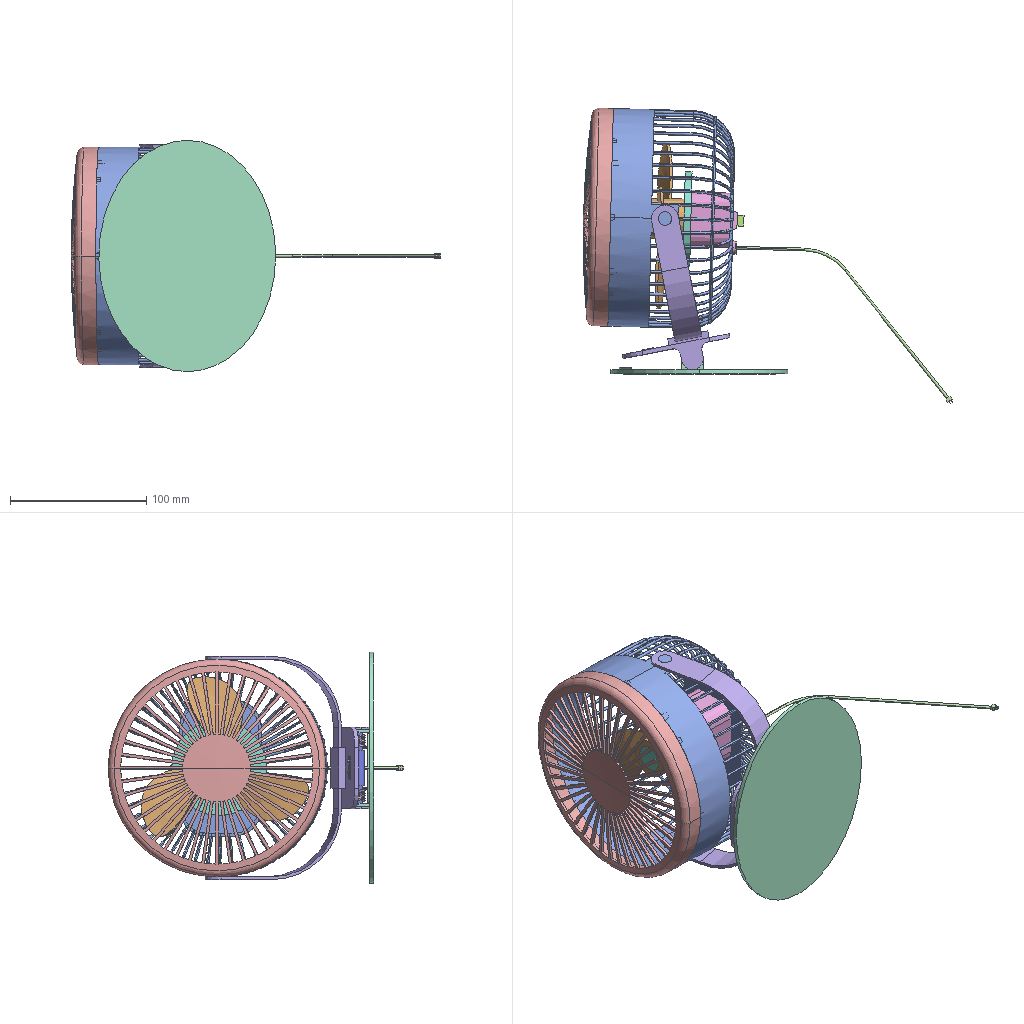Assembly | SolidWorks | 12 different items | 12 placed | box 272 x 217 x 170 mm
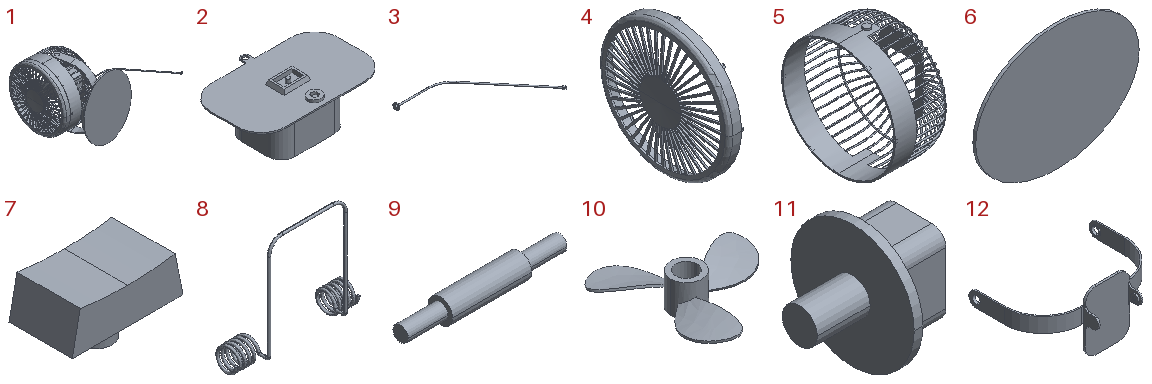Parts list (item | name | quantity | size | volume | features):
1 | (subassembly) | x1 | 271.678 x 217.243 x 170 mm | 282598 mm3 | features CompositeCurve 4
2 | - | x1 | 96 x 63 x 34 mm | 14984 mm3 | features ICE 4, Fillet 2, Extrusion 1
3 | - | x1 | 164.795 x 115.719 x 10 mm | 796.943 mm3 | features ICE 2, Revolution 1, Sweep 1
4 | - | x1 | 23 x 160 x 160 mm | 32777 mm3 | features ICE 2, CirPattern 1, Fillet 1, Revolution 1, Shell 1
5 | - | x1 | 90 x 160 x 164 mm | 49564 mm3 | features ICE 8, Revolution 3, MirrorSolid 2, CirPattern 1, CombineBodies 1, MirrorPattern 1, MoveCopyBody 1, Sweep 1
6 | - | x1 | 170 x 19 x 130 mm | 53107 mm3 | features ICE 6, Extrusion 1, SweepCut 1
7 | - | x1 | 14 x 8 x 8 mm | 507.497 mm3 | features Extrusion 1, ICE 1
8 | - | x1 | 48.997 x 12.996 x 44.996 mm | 285.893 mm3 | features 3DProfileFeature 2, Helix 1, MirrorPattern 1, Sweep 1
9 | - | x1 | 52 x 8 x 8 mm | 1817 mm3 | features Revolution 1
10 | - | x1 | 117.735 x 123.352 x 30 mm | 21277 mm3 | features BlendRefSurface 1, CirPattern 1, CombineBodies 1, Extrusion 1, ICE 1, Thicken 1, TrimRefSurface 1
11 | - | x1 | 65 x 70 x 70 mm | 76699 mm3 | features Extrusion 1, Revolution 1
12 | - | x1 | 164 x 123 x 80 mm | 30766 mm3 | features ICE 13, Extrusion 1, Fillet 1
Mates (type | each side: item.copy, entity, surface, feature):
Concentric | 4.1 face cylinder Revolve1 | 5.1 face cylinder Revolve1
Coincident | 4.1 face plane Revolve1 | 5.1 face plane Revolve1
Coincident | 4.1 plane | 5.1 plane
Coincident | 5.1 face plane Cut-Extrude5 | 2.1 face plane Boss-Extrude1
Concentric | 5.1 edge | 2.1 edge | 2 times
Concentric | 7.1 face cylinder Boss-Extrude2 | 2.1 face cylinder Cut-Extrude1
Coincident | 7.1 face plane Boss-Extrude2 | 2.1 face plane Cut-Extrude1
Parallel | 7.1 face plane Boss-Extrude1 | 2.1 face plane Cut-Extrude1
Coincident | 2.1 face plane Boss-Extrude3 | 11.1 face plane Boss-Extrude1 | 2 times
Coincident | 2.1 face plane Boss-Extrude1 | 11.1 face plane Boss-Extrude1
Coincident | 11.1 face plane Revolve1 | 10.1 face plane Boss-Extrude1
Concentric | 11.1 face cylinder Revolve1 | 10.1 face cylinder Cut-Extrude1
Concentric | 5.1 face cylinder Boss-Extrude4 | 12.1 face cylinder Cut-Extrude1
Coincident | 4.1 plane | 12.1 plane
Coincident | 6.1 plane | assembly plane | 3 times
Concentric | 12.1 face cylinder Boss-Extrude11 | 6.1 face cylinder Boss-Extrude3
Coincident | 12.1 face plane Boss-Extrude9 | 6.1 face plane Boss-Extrude3
Concentric | 6.1 face cylinder Cut-Sweep1 | 8.1 face cylinder Mirror1
Concentric | 6.1 face cylinder Cut-Sweep1 | 8.1 face cylinder Sweep1
Concentric | 12.1 face cylinder Cut-Extrude4 | 9.1 face cylinder Revolve1
Coincident | 9.1 plane | assembly plane
Concentric | 2.1 face cylinder Boss-Extrude4 | 3.1 face cylinder Sweep1
Coincident | 2.1 face plane Boss-Extrude1 | 3.1 face plane Revolve1
Coincident | 3.1 plane | assembly plane